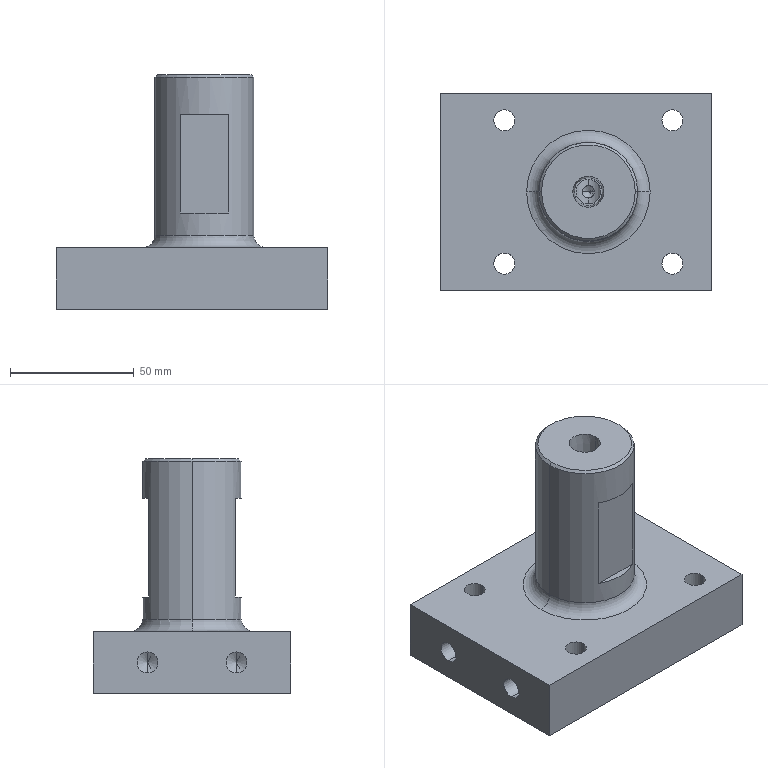Part | SolidWorks | features HoleWzd 5, ICE 4, Chamfer 1, Extrusion 1, Fillet 1, RevCut 1 | 1 solid | 54 faces | box 110 x 80 x 95 mm | volume 289106 mm3 | cylinder 24 | cone 14 | plane 14 | torus 2 | commonest cylinder face diameters 8.5 x12 5 x4 11.8 x4 10 x2 40 x2